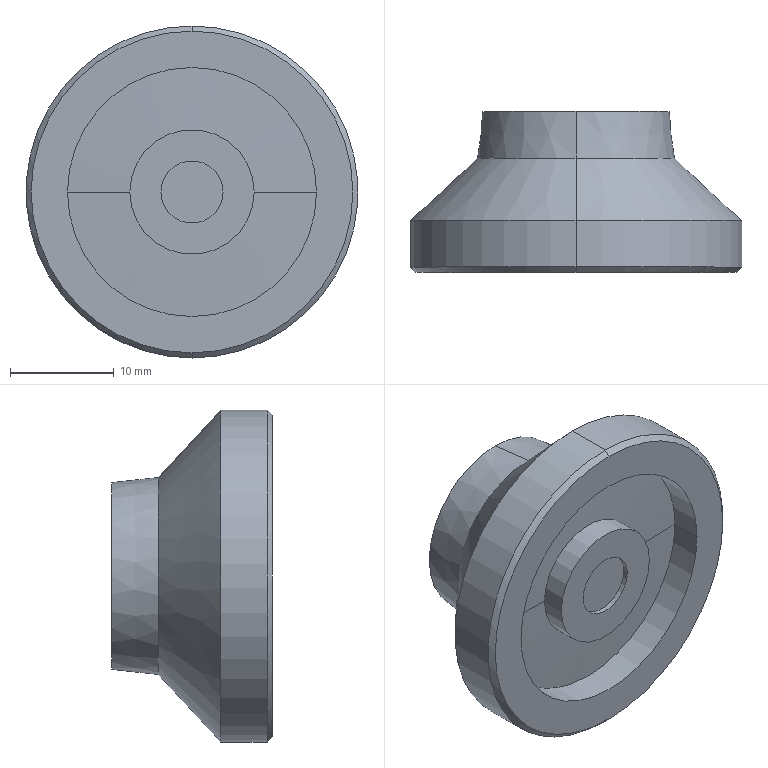Part | STEP file | 343.8-32-M8-63-A | 1 solid | 28 faces | box 32 x 15.5 x 32 mm | volume 6505 mm3 | cone 10 | cylinder 8 | torus 4 | plane 4 | sphere 2 | commonest cylinder face diameters 6 x2 12 x2 24 x2 32 x2